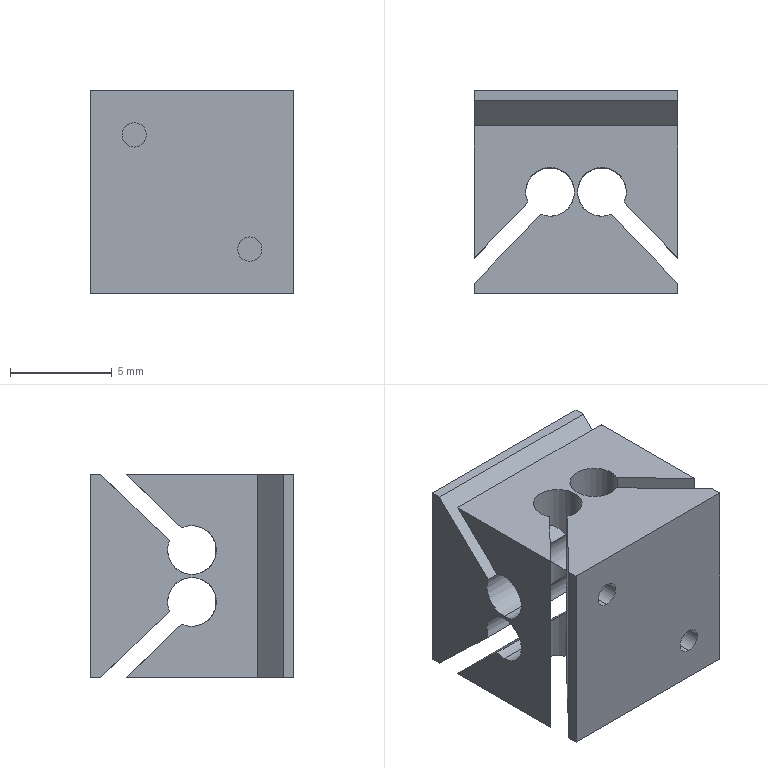Part | SolidWorks | features ICE 4, Extrusion 1 | 1 solid | 80 faces | box 10 x 10 x 10 mm | volume 690.684 mm3 | cylinder 56 | plane 24 | commonest cylinder face diameters 2.4 x44 2 x8 1.2 x4